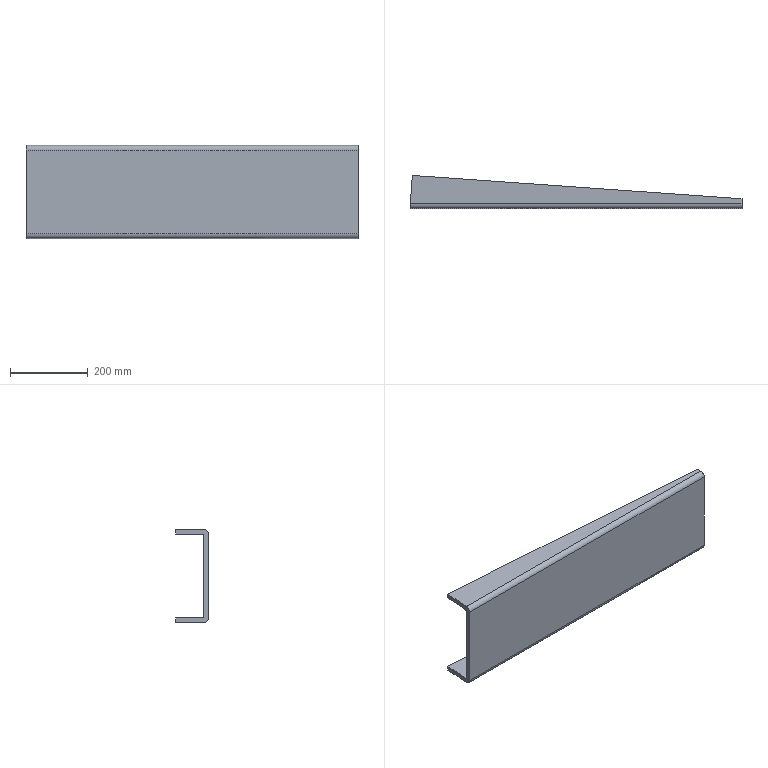Part | SolidWorks | features ICE 4, Fillet 2, Extrusion 1, Shell 1 | 1 solid | 14 faces | box 856 x 85 x 240 mm | volume 3296184 mm3 | plane 10 | cylinder 4 | commonest cylinder face diameters 6 x2 24 x2
STEP:
#1=CARTESIAN_POINT('',(425.,-30.5,240.));
#2=VERTEX_POINT('',#1);
#3=CARTESIAN_POINT('',(425.,-17.5,240.));
#4=VERTEX_POINT('',#3);
#5=CARTESIAN_POINT('',(425.,42.5,240.));
#6=DIRECTION('',(0.,1.,0.));
#7=VECTOR('',#6,1000.);
#8=LINE('',#5,#7);
#9=EDGE_CURVE('',#2,#4,#8,.T.);
#10=ORIENTED_EDGE('',*,*,#9,.F.);
#11=CARTESIAN_POINT('',(425.,-42.5,228.));
#12=VERTEX_POINT('',#11);
#13=CARTESIAN_POINT('',(425.,-30.5,228.));
#14=DIRECTION('',(1.,0.,0.));
#15=DIRECTION('',(0.,0.,1.));
#16=AXIS2_PLACEMENT_3D('',#13,#14,#15);
#17=CIRCLE('',#16,12.);
#18=EDGE_CURVE('',#2,#12,#17,.T.);
#19=ORIENTED_EDGE('',*,*,#18,.T.);
#20=CARTESIAN_POINT('',(425.,-42.5,12.));
#21=VERTEX_POINT('',#20);
#22=CARTESIAN_POINT('',(425.,-42.5,240.));
#23=DIRECTION('',(0.,0.,-1.));
#24=VECTOR('',#23,1000.);
#25=LINE('',#22,#24);
#26=EDGE_CURVE('',#12,#21,#25,.T.);
#27=ORIENTED_EDGE('',*,*,#26,.T.);
#28=CARTESIAN_POINT('',(425.,-30.5,0.));
#29=VERTEX_POINT('',#28);
#30=CARTESIAN_POINT('',(425.,-30.5,12.));
#31=DIRECTION('',(1.,0.,0.));
#32=DIRECTION('',(0.,0.,1.));
#33=AXIS2_PLACEMENT_3D('',#30,#31,#32);
#34=CIRCLE('',#33,12.);
#35=EDGE_CURVE('',#21,#29,#34,.T.);
#36=ORIENTED_EDGE('',*,*,#35,.T.);
#37=CARTESIAN_POINT('',(425.,-17.5,0.));
#38=VERTEX_POINT('',#37);
#39=CARTESIAN_POINT('',(425.,42.5,0.));
#40=DIRECTION('',(0.,1.,0.));
#41=VECTOR('',#40,1000.);
#42=LINE('',#39,#41);
#43=EDGE_CURVE('',#29,#38,#42,.T.);
#44=ORIENTED_EDGE('',*,*,#43,.T.);
#45=CARTESIAN_POINT('',(425.,-17.5,12.));
#46=VERTEX_POINT('',#45);
#47=CARTESIAN_POINT('',(425.,-17.5,0.));
#48=DIRECTION('',(0.,0.,1.));
#49=VECTOR('',#48,1000.);
#50=LINE('',#47,#49);
#51=EDGE_CURVE('',#38,#46,#50,.T.);
#52=ORIENTED_EDGE('',*,*,#51,.T.);
#53=CARTESIAN_POINT('',(425.,-27.5,12.));
#54=VERTEX_POINT('',#53);
#55=CARTESIAN_POINT('',(425.,0.,12.));
#56=DIRECTION('',(0.,1.,0.));
#57=VECTOR('',#56,1000.);
#58=LINE('',#55,#57);
#59=EDGE_CURVE('',#54,#46,#58,.T.);
#60=ORIENTED_EDGE('',*,*,#59,.F.);
#61=CARTESIAN_POINT('',(425.,-30.5,15.));
#62=VERTEX_POINT('',#61);
#63=CARTESIAN_POINT('',(425.,-27.5,15.));
#64=DIRECTION('',(-1.,0.,0.));
#65=DIRECTION('',(0.,0.,1.));
#66=AXIS2_PLACEMENT_3D('',#63,#64,#65);
#67=CIRCLE('',#66,3.);
#68=EDGE_CURVE('',#54,#62,#67,.T.);
#69=ORIENTED_EDGE('',*,*,#68,.T.);
#70=CARTESIAN_POINT('',(425.,-30.5,225.));
#71=VERTEX_POINT('',#70);
#72=CARTESIAN_POINT('',(425.,-30.5,240.));
#73=DIRECTION('',(0.,0.,-1.));
#74=VECTOR('',#73,1000.);
#75=LINE('',#72,#74);
#76=EDGE_CURVE('',#71,#62,#75,.T.);
#77=ORIENTED_EDGE('',*,*,#76,.F.);
#78=CARTESIAN_POINT('',(425.,-27.5,228.));
#79=VERTEX_POINT('',#78);
#80=CARTESIAN_POINT('',(425.,-27.5,225.));
#81=DIRECTION('',(-1.,0.,0.));
#82=DIRECTION('',(0.,0.,1.));
#83=AXIS2_PLACEMENT_3D('',#80,#81,#82);
#84=CIRCLE('',#83,3.);
#85=EDGE_CURVE('',#71,#79,#84,.T.);
#86=ORIENTED_EDGE('',*,*,#85,.T.);
#87=CARTESIAN_POINT('',(425.,-17.5,228.));
#88=VERTEX_POINT('',#87);
#89=CARTESIAN_POINT('',(425.,0.,228.));
#90=DIRECTION('',(0.,1.,0.));
#91=VECTOR('',#90,1000.);
#92=LINE('',#89,#91);
#93=EDGE_CURVE('',#79,#88,#92,.T.);
#94=ORIENTED_EDGE('',*,*,#93,.T.);
#95=CARTESIAN_POINT('',(425.,-17.5,0.));
#96=DIRECTION('',(0.,0.,1.));
#97=VECTOR('',#96,1000.);
#98=LINE('',#95,#97);
#99=EDGE_CURVE('',#88,#4,#98,.T.);
#100=ORIENTED_EDGE('',*,*,#99,.T.);
#101=EDGE_LOOP('',(#10,#19,#27,#36,#44,#52,#60,#69,#77,#86,#94,#100));
#102=FACE_OUTER_BOUND('',#101,.T.);
#103=CARTESIAN_POINT('',(425.,42.5,240.));
#104=DIRECTION('',(-1.,0.,0.));
#105=DIRECTION('',(0.,0.,1.));
#106=AXIS2_PLACEMENT_3D('',#103,#104,#105);
#107=PLANE('',#106);
#108=ADVANCED_FACE('',(#102),#107,.F.);
#109=CARTESIAN_POINT('',(-425.,42.5,12.));
#110=VERTEX_POINT('',#109);
#111=CARTESIAN_POINT('',(-425.,42.5,12.));
#112=DIRECTION('',(-0.9975,0.07041,0.));
#113=VECTOR('',#112,1000.);
#114=LINE('',#111,#113);
#115=EDGE_CURVE('',#46,#110,#114,.T.);
#116=ORIENTED_EDGE('',*,*,#115,.F.);
#117=ORIENTED_EDGE('',*,*,#51,.F.);
#118=CARTESIAN_POINT('',(-425.,42.5,0.));
#119=VERTEX_POINT('',#118);
#120=CARTESIAN_POINT('',(-425.,42.5,0.));
#121=DIRECTION('',(0.9975,-0.07041,0.));
#122=VECTOR('',#121,1000.);
#123=LINE('',#120,#122);
#124=EDGE_CURVE('',#119,#38,#123,.T.);
#125=ORIENTED_EDGE('',*,*,#124,.F.);
#126=CARTESIAN_POINT('',(-425.,42.5,240.));
#127=DIRECTION('',(0.,0.,-1.));
#128=VECTOR('',#127,1000.);
#129=LINE('',#126,#128);
#130=EDGE_CURVE('',#110,#119,#129,.T.);
#131=ORIENTED_EDGE('',*,*,#130,.F.);
#132=EDGE_LOOP('',(#116,#117,#125,#131));
#133=FACE_OUTER_BOUND('',#132,.T.);
#134=CARTESIAN_POINT('',(-425.,42.5,0.));
#135=DIRECTION('',(-0.07041,-0.9975,0.));
#136=DIRECTION('',(0.9975,-0.07041,0.));
#137=AXIS2_PLACEMENT_3D('',#134,#135,#136);
#138=PLANE('',#137);
#139=ADVANCED_FACE('',(#133),#138,.F.);
#140=CARTESIAN_POINT('',(-425.,42.5,228.));
#141=VERTEX_POINT('',#140);
#142=CARTESIAN_POINT('',(-425.,42.5,228.));
#143=DIRECTION('',(0.9975,-0.07041,0.));
#144=VECTOR('',#143,1000.);
#145=LINE('',#142,#144);
#146=EDGE_CURVE('',#141,#88,#145,.T.);
#147=ORIENTED_EDGE('',*,*,#146,.F.);
#148=CARTESIAN_POINT('',(-425.,42.5,240.));
#149=VERTEX_POINT('',#148);
#150=CARTESIAN_POINT('',(-425.,42.5,240.));
#151=DIRECTION('',(0.,0.,-1.));
#152=VECTOR('',#151,1000.);
#153=LINE('',#150,#152);
#154=EDGE_CURVE('',#149,#141,#153,.T.);
#155=ORIENTED_EDGE('',*,*,#154,.F.);
#156=CARTESIAN_POINT('',(-425.,42.5,240.));
#157=DIRECTION('',(0.9975,-0.07041,0.));
#158=VECTOR('',#157,1000.);
#159=LINE('',#156,#158);
#160=EDGE_CURVE('',#149,#4,#159,.T.);
#161=ORIENTED_EDGE('',*,*,#160,.T.);
#162=ORIENTED_EDGE('',*,*,#99,.F.);
#163=EDGE_LOOP('',(#147,#155,#161,#162));
#164=FACE_OUTER_BOUND('',#163,.T.);
#165=CARTESIAN_POINT('',(-425.,42.5,0.));
#166=DIRECTION('',(-0.07041,-0.9975,0.));
#167=DIRECTION('',(0.9975,-0.07041,0.));
#168=AXIS2_PLACEMENT_3D('',#165,#166,#167);
#169=PLANE('',#168);
#170=ADVANCED_FACE('',(#164),#169,.F.);
#171=ORIENTED_EDGE('',*,*,#26,.F.);
#172=CARTESIAN_POINT('',(-431.,-42.5,228.));
#173=VERTEX_POINT('',#172);
#174=CARTESIAN_POINT('',(425.,-42.5,228.));
#175=DIRECTION('',(-1.,0.,0.));
#176=VECTOR('',#175,1000.);
#177=LINE('',#174,#176);
#178=EDGE_CURVE('',#12,#173,#177,.T.);
#179=ORIENTED_EDGE('',*,*,#178,.T.);
#180=CARTESIAN_POINT('',(-431.,-42.5,12.));
#181=VERTEX_POINT('',#180);
#182=CARTESIAN_POINT('',(-431.,-42.5,240.));
#183=DIRECTION('',(0.,0.,-1.));
#184=VECTOR('',#183,1000.);
#185=LINE('',#182,#184);
#186=EDGE_CURVE('',#173,#181,#185,.T.);
#187=ORIENTED_EDGE('',*,*,#186,.T.);
#188=CARTESIAN_POINT('',(425.,-42.5,12.));
#189=DIRECTION('',(1.,0.,0.));
#190=VECTOR('',#189,1000.);
#191=LINE('',#188,#190);
#192=EDGE_CURVE('',#181,#21,#191,.T.);
#193=ORIENTED_EDGE('',*,*,#192,.T.);
#194=EDGE_LOOP('',(#171,#179,#187,#193));
#195=FACE_OUTER_BOUND('',#194,.T.);
#196=CARTESIAN_POINT('',(425.,-42.5,240.));
#197=DIRECTION('',(0.,1.,0.));
#198=DIRECTION('',(-1.,0.,0.));
#199=AXIS2_PLACEMENT_3D('',#196,#197,#198);
#200=PLANE('',#199);
#201=ADVANCED_FACE('',(#195),#200,.F.);
#202=CARTESIAN_POINT('',(-430.153,-30.5,240.));
#203=VERTEX_POINT('',#202);
#204=CARTESIAN_POINT('',(-425.,42.5,240.));
#205=DIRECTION('',(0.07041,0.9975,0.));
#206=VECTOR('',#205,1000.);
#207=LINE('',#204,#206);
#208=EDGE_CURVE('',#203,#149,#207,.T.);
#209=ORIENTED_EDGE('',*,*,#208,.F.);
#210=CARTESIAN_POINT('',(0.,-30.5,240.));
#211=DIRECTION('',(1.,0.,0.));
#212=VECTOR('',#211,1000.);
#213=LINE('',#210,#212);
#214=EDGE_CURVE('',#203,#2,#213,.T.);
#215=ORIENTED_EDGE('',*,*,#214,.T.);
#216=ORIENTED_EDGE('',*,*,#9,.T.);
#217=ORIENTED_EDGE('',*,*,#160,.F.);
#218=EDGE_LOOP('',(#209,#215,#216,#217));
#219=FACE_OUTER_BOUND('',#218,.T.);
#220=CARTESIAN_POINT('',(0.,0.,240.));
#221=DIRECTION('',(0.,0.,-1.));
#222=DIRECTION('',(-1.,0.,0.));
#223=AXIS2_PLACEMENT_3D('',#220,#221,#222);
#224=PLANE('',#223);
#225=ADVANCED_FACE('',(#219),#224,.F.);
#226=ORIENTED_EDGE('',*,*,#43,.F.);
#227=CARTESIAN_POINT('',(-430.153,-30.5,0.));
#228=VERTEX_POINT('',#227);
#229=CARTESIAN_POINT('',(-431.,-30.5,0.));
#230=DIRECTION('',(-1.,0.,0.));
#231=VECTOR('',#230,1000.);
#232=LINE('',#229,#231);
#233=EDGE_CURVE('',#29,#228,#232,.T.);
#234=ORIENTED_EDGE('',*,*,#233,.T.);
#235=CARTESIAN_POINT('',(-425.,42.5,0.));
#236=DIRECTION('',(0.07041,0.9975,0.));
#237=VECTOR('',#236,1000.);
#238=LINE('',#235,#237);
#239=EDGE_CURVE('',#228,#119,#238,.T.);
#240=ORIENTED_EDGE('',*,*,#239,.T.);
#241=ORIENTED_EDGE('',*,*,#124,.T.);
#242=EDGE_LOOP('',(#226,#234,#240,#241));
#243=FACE_OUTER_BOUND('',#242,.T.);
#244=CARTESIAN_POINT('',(0.,0.,0.));
#245=DIRECTION('',(0.,0.,-1.));
#246=DIRECTION('',(-1.,0.,0.));
#247=AXIS2_PLACEMENT_3D('',#244,#245,#246);
#248=PLANE('',#247);
#249=ADVANCED_FACE('',(#243),#248,.T.);
#250=ORIENTED_EDGE('',*,*,#76,.T.);
#251=CARTESIAN_POINT('',(-430.153,-30.5,15.));
#252=VERTEX_POINT('',#251);
#253=CARTESIAN_POINT('',(425.,-30.5,15.));
#254=DIRECTION('',(-1.,0.,0.));
#255=VECTOR('',#254,1000.);
#256=LINE('',#253,#255);
#257=EDGE_CURVE('',#62,#252,#256,.T.);
#258=ORIENTED_EDGE('',*,*,#257,.T.);
#259=CARTESIAN_POINT('',(-430.153,-30.5,225.));
#260=VERTEX_POINT('',#259);
#261=CARTESIAN_POINT('',(-430.153,-30.5,240.));
#262=DIRECTION('',(0.,0.,1.));
#263=VECTOR('',#262,1000.);
#264=LINE('',#261,#263);
#265=EDGE_CURVE('',#252,#260,#264,.T.);
#266=ORIENTED_EDGE('',*,*,#265,.T.);
#267=CARTESIAN_POINT('',(425.,-30.5,225.));
#268=DIRECTION('',(1.,0.,0.));
#269=VECTOR('',#268,1000.);
#270=LINE('',#267,#269);
#271=EDGE_CURVE('',#260,#71,#270,.T.);
#272=ORIENTED_EDGE('',*,*,#271,.T.);
#273=EDGE_LOOP('',(#250,#258,#266,#272));
#274=FACE_OUTER_BOUND('',#273,.T.);
#275=CARTESIAN_POINT('',(425.,-30.5,240.));
#276=DIRECTION('',(0.,1.,0.));
#277=DIRECTION('',(-1.,0.,0.));
#278=AXIS2_PLACEMENT_3D('',#275,#276,#277);
#279=PLANE('',#278);
#280=ADVANCED_FACE('',(#274),#279,.T.);
#281=ORIENTED_EDGE('',*,*,#93,.F.);
#282=CARTESIAN_POINT('',(-429.941,-27.5,228.));
#283=VERTEX_POINT('',#282);
#284=CARTESIAN_POINT('',(-425.,-27.5,228.));
#285=DIRECTION('',(-1.,0.,0.));
#286=VECTOR('',#285,1000.);
#287=LINE('',#284,#286);
#288=EDGE_CURVE('',#79,#283,#287,.T.);
#289=ORIENTED_EDGE('',*,*,#288,.T.);
#290=CARTESIAN_POINT('',(-425.,42.5,228.));
#291=DIRECTION('',(0.07041,0.9975,0.));
#292=VECTOR('',#291,1000.);
#293=LINE('',#290,#292);
#294=EDGE_CURVE('',#283,#141,#293,.T.);
#295=ORIENTED_EDGE('',*,*,#294,.T.);
#296=ORIENTED_EDGE('',*,*,#146,.T.);
#297=EDGE_LOOP('',(#281,#289,#295,#296));
#298=FACE_OUTER_BOUND('',#297,.T.);
#299=CARTESIAN_POINT('',(0.,0.,228.));
#300=DIRECTION('',(0.,0.,-1.));
#301=DIRECTION('',(-1.,0.,0.));
#302=AXIS2_PLACEMENT_3D('',#299,#300,#301);
#303=PLANE('',#302);
#304=ADVANCED_FACE('',(#298),#303,.T.);
#305=ORIENTED_EDGE('',*,*,#115,.T.);
#306=CARTESIAN_POINT('',(-429.941,-27.5,12.));
#307=VERTEX_POINT('',#306);
#308=CARTESIAN_POINT('',(-425.,42.5,12.));
#309=DIRECTION('',(-0.07041,-0.9975,0.));
#310=VECTOR('',#309,1000.);
#311=LINE('',#308,#310);
#312=EDGE_CURVE('',#110,#307,#311,.T.);
#313=ORIENTED_EDGE('',*,*,#312,.T.);
#314=CARTESIAN_POINT('',(0.,-27.5,12.));
#315=DIRECTION('',(1.,0.,0.));
#316=VECTOR('',#315,1000.);
#317=LINE('',#314,#316);
#318=EDGE_CURVE('',#307,#54,#317,.T.);
#319=ORIENTED_EDGE('',*,*,#318,.T.);
#320=ORIENTED_EDGE('',*,*,#59,.T.);
#321=EDGE_LOOP('',(#305,#313,#319,#320));
#322=FACE_OUTER_BOUND('',#321,.T.);
#323=CARTESIAN_POINT('',(0.,0.,12.));
#324=DIRECTION('',(0.,0.,-1.));
#325=DIRECTION('',(-1.,0.,0.));
#326=AXIS2_PLACEMENT_3D('',#323,#324,#325);
#327=PLANE('',#326);
#328=ADVANCED_FACE('',(#322),#327,.F.);
#329=ORIENTED_EDGE('',*,*,#294,.F.);
#330=CARTESIAN_POINT('',(-430.153,-30.5,225.));
#331=CARTESIAN_POINT('',(-430.153,-30.5,226.757));
#332=CARTESIAN_POINT('',(-430.065,-29.257,228.));
#333=CARTESIAN_POINT('',(-429.941,-27.5,228.));
#334=(BOUNDED_CURVE()B_SPLINE_CURVE(3,(#330,#331,#332,#333),.UNSPECIFIED.,.F.,.F.)B_SPLINE_CURVE_WITH_KNOTS((4,4),(3.142,4.712),.UNSPECIFIED.)CURVE()GEOMETRIC_REPRESENTATION_ITEM()RATIONAL_B_SPLINE_CURVE((1.,0.8047,0.8047,1.))REPRESENTATION_ITEM(''));
#335=EDGE_CURVE('',#260,#283,#334,.T.);
#336=ORIENTED_EDGE('',*,*,#335,.F.);
#337=ORIENTED_EDGE('',*,*,#265,.F.);
#338=CARTESIAN_POINT('',(-429.941,-27.5,12.));
#339=CARTESIAN_POINT('',(-430.065,-29.257,12.));
#340=CARTESIAN_POINT('',(-430.153,-30.5,13.243));
#341=CARTESIAN_POINT('',(-430.153,-30.5,15.));
#342=(BOUNDED_CURVE()B_SPLINE_CURVE(3,(#338,#339,#340,#341),.UNSPECIFIED.,.F.,.F.)B_SPLINE_CURVE_WITH_KNOTS((4,4),(1.571,3.142),.UNSPECIFIED.)CURVE()GEOMETRIC_REPRESENTATION_ITEM()RATIONAL_B_SPLINE_CURVE((1.,0.8047,0.8047,1.))REPRESENTATION_ITEM(''));
#343=EDGE_CURVE('',#307,#252,#342,.T.);
#344=ORIENTED_EDGE('',*,*,#343,.F.);
#345=ORIENTED_EDGE('',*,*,#312,.F.);
#346=ORIENTED_EDGE('',*,*,#130,.T.);
#347=ORIENTED_EDGE('',*,*,#239,.F.);
#348=CARTESIAN_POINT('',(-430.153,-30.5,0.));
#349=CARTESIAN_POINT('',(-430.649,-37.529,0.));
#350=CARTESIAN_POINT('',(-431.,-42.5,4.971));
#351=CARTESIAN_POINT('',(-431.,-42.5,12.));
#352=(BOUNDED_CURVE()B_SPLINE_CURVE(3,(#348,#349,#350,#351),.UNSPECIFIED.,.F.,.F.)B_SPLINE_CURVE_WITH_KNOTS((4,4),(4.712,6.283),.UNSPECIFIED.)CURVE()GEOMETRIC_REPRESENTATION_ITEM()RATIONAL_B_SPLINE_CURVE((1.,0.8047,0.8047,1.))REPRESENTATION_ITEM(''));
#353=EDGE_CURVE('',#228,#181,#352,.T.);
#354=ORIENTED_EDGE('',*,*,#353,.T.);
#355=ORIENTED_EDGE('',*,*,#186,.F.);
#356=CARTESIAN_POINT('',(-431.,-42.5,228.));
#357=CARTESIAN_POINT('',(-431.,-42.5,235.029));
#358=CARTESIAN_POINT('',(-430.649,-37.529,240.));
#359=CARTESIAN_POINT('',(-430.153,-30.5,240.));
#360=(BOUNDED_CURVE()B_SPLINE_CURVE(3,(#356,#357,#358,#359),.UNSPECIFIED.,.F.,.T.)B_SPLINE_CURVE_WITH_KNOTS((4,4),(3.142,4.712),.UNSPECIFIED.)CURVE()GEOMETRIC_REPRESENTATION_ITEM()RATIONAL_B_SPLINE_CURVE((1.,0.8047,0.8047,1.))REPRESENTATION_ITEM(''));
#361=EDGE_CURVE('',#173,#203,#360,.T.);
#362=ORIENTED_EDGE('',*,*,#361,.T.);
#363=ORIENTED_EDGE('',*,*,#208,.T.);
#364=ORIENTED_EDGE('',*,*,#154,.T.);
#365=EDGE_LOOP('',(#329,#336,#337,#344,#345,#346,#347,#354,#355,#362,#363,#364));
#366=FACE_OUTER_BOUND('',#365,.T.);
#367=CARTESIAN_POINT('',(-425.,42.5,240.));
#368=DIRECTION('',(-0.9975,0.07041,0.));
#369=DIRECTION('',(-0.07041,-0.9975,0.));
#370=AXIS2_PLACEMENT_3D('',#367,#368,#369);
#371=PLANE('',#370);
#372=ADVANCED_FACE('',(#366),#371,.T.);
#373=ORIENTED_EDGE('',*,*,#361,.F.);
#374=ORIENTED_EDGE('',*,*,#178,.F.);
#375=ORIENTED_EDGE('',*,*,#18,.F.);
#376=ORIENTED_EDGE('',*,*,#214,.F.);
#377=EDGE_LOOP('',(#373,#374,#375,#376));
#378=FACE_OUTER_BOUND('',#377,.T.);
#379=CARTESIAN_POINT('',(0.,-30.5,228.));
#380=DIRECTION('',(1.,0.,0.));
#381=DIRECTION('',(0.,1.,0.));
#382=AXIS2_PLACEMENT_3D('',#379,#380,#381);
#383=CYLINDRICAL_SURFACE('',#382,12.);
#384=ADVANCED_FACE('',(#378),#383,.T.);
#385=ORIENTED_EDGE('',*,*,#353,.F.);
#386=ORIENTED_EDGE('',*,*,#233,.F.);
#387=ORIENTED_EDGE('',*,*,#35,.F.);
#388=ORIENTED_EDGE('',*,*,#192,.F.);
#389=EDGE_LOOP('',(#385,#386,#387,#388));
#390=FACE_OUTER_BOUND('',#389,.T.);
#391=CARTESIAN_POINT('',(425.,-30.5,12.));
#392=DIRECTION('',(-1.,0.,0.));
#393=DIRECTION('',(0.,-1.,0.));
#394=AXIS2_PLACEMENT_3D('',#391,#392,#393);
#395=CYLINDRICAL_SURFACE('',#394,12.);
#396=ADVANCED_FACE('',(#390),#395,.T.);
#397=ORIENTED_EDGE('',*,*,#318,.F.);
#398=ORIENTED_EDGE('',*,*,#343,.T.);
#399=ORIENTED_EDGE('',*,*,#257,.F.);
#400=ORIENTED_EDGE('',*,*,#68,.F.);
#401=EDGE_LOOP('',(#397,#398,#399,#400));
#402=FACE_OUTER_BOUND('',#401,.T.);
#403=CARTESIAN_POINT('',(0.,-27.5,15.));
#404=DIRECTION('',(1.,0.,0.));
#405=DIRECTION('',(0.,1.,0.));
#406=AXIS2_PLACEMENT_3D('',#403,#404,#405);
#407=CYLINDRICAL_SURFACE('',#406,3.);
#408=ADVANCED_FACE('',(#402),#407,.F.);
#409=ORIENTED_EDGE('',*,*,#271,.F.);
#410=ORIENTED_EDGE('',*,*,#335,.T.);
#411=ORIENTED_EDGE('',*,*,#288,.F.);
#412=ORIENTED_EDGE('',*,*,#85,.F.);
#413=EDGE_LOOP('',(#409,#410,#411,#412));
#414=FACE_OUTER_BOUND('',#413,.T.);
#415=CARTESIAN_POINT('',(425.,-27.5,225.));
#416=DIRECTION('',(-1.,0.,0.));
#417=DIRECTION('',(0.,-1.,0.));
#418=AXIS2_PLACEMENT_3D('',#415,#416,#417);
#419=CYLINDRICAL_SURFACE('',#418,3.);
#420=ADVANCED_FACE('',(#414),#419,.F.);
#421=CLOSED_SHELL('',(#108,#139,#170,#201,#225,#249,#280,#304,#328,#372,#384,#396,#408,#420));
#422=MANIFOLD_SOLID_BREP('',#421);
#423=CARTESIAN_POINT('',(0.,0.,0.));
#424=DIRECTION('',(0.,0.,1.));
#425=DIRECTION('',(1.,0.,0.));
#426=AXIS2_PLACEMENT_3D('',#423,#424,#425);
#427=(LENGTH_UNIT()NAMED_UNIT(*)SI_UNIT(.MILLI.,.METRE.));
#428=UNCERTAINTY_MEASURE_WITH_UNIT(LENGTH_MEASURE(0.00001),#427,'','');
#429=(NAMED_UNIT(*)PLANE_ANGLE_UNIT()SI_UNIT($,.RADIAN.));
#430=(NAMED_UNIT(*)SI_UNIT($,.STERADIAN.)SOLID_ANGLE_UNIT());
#431=(GEOMETRIC_REPRESENTATION_CONTEXT(3)GLOBAL_UNCERTAINTY_ASSIGNED_CONTEXT((#428))GLOBAL_UNIT_ASSIGNED_CONTEXT((#427,#429,#430))REPRESENTATION_CONTEXT('',''));
#432=ADVANCED_BREP_SHAPE_REPRESENTATION('',(#422,#426),#431);